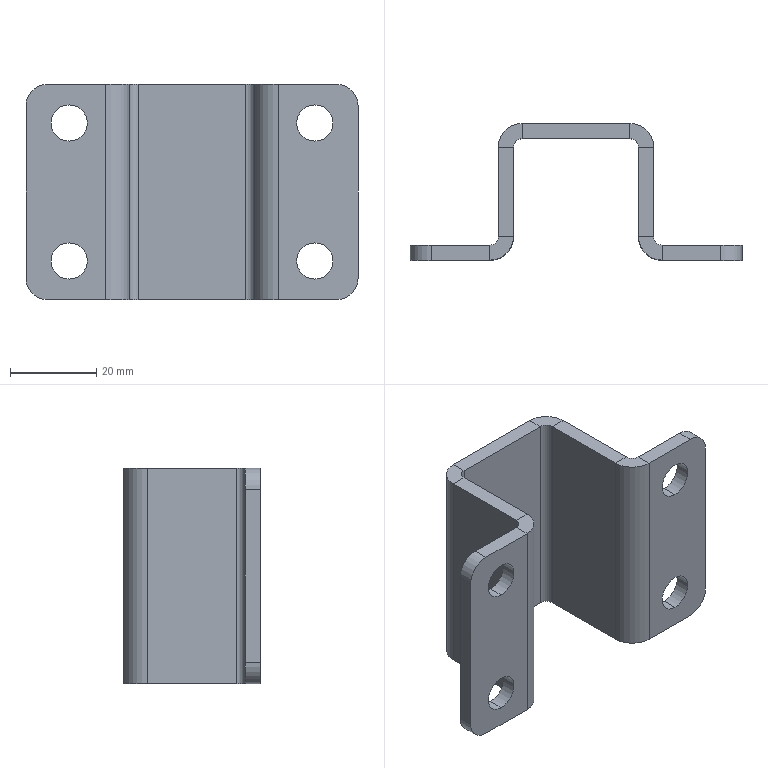Part | STEP file | ABRAZADERA a | 1 solid | 50 faces | box 77 x 31.7 x 50 mm | volume 21367 mm3 | plane 30 | cylinder 20 | commonest cylinder face diameters 8.4 x8 4 x4 10 x4 11 x4
STEP:
#1=CARTESIAN_POINT('',(-28.5,-13.7,11.8));
#2=VERTEX_POINT('',#1);
#3=CARTESIAN_POINT('',(-28.5,-13.7,20.2));
#4=VERTEX_POINT('',#3);
#5=CARTESIAN_POINT('',(-28.5,-13.7,16.));
#6=DIRECTION('',(0.,1.,0.));
#7=DIRECTION('',(-1.,0.,0.));
#8=AXIS2_PLACEMENT_3D('',#5,#6,#7);
#9=CIRCLE('',#8,4.2);
#10=EDGE_CURVE('',#2,#4,#9,.T.);
#11=ORIENTED_EDGE('',*,*,#10,.F.);
#12=CARTESIAN_POINT('',(-28.5,-10.2,11.8));
#13=VERTEX_POINT('',#12);
#14=CARTESIAN_POINT('',(-28.5,-10.2,11.8));
#15=DIRECTION('',(0.,1.,0.));
#16=VECTOR('',#15,1000.);
#17=LINE('',#14,#16);
#18=EDGE_CURVE('',#2,#13,#17,.T.);
#19=ORIENTED_EDGE('',*,*,#18,.T.);
#20=CARTESIAN_POINT('',(-28.5,-10.2,20.2));
#21=VERTEX_POINT('',#20);
#22=CARTESIAN_POINT('',(-28.5,-10.2,16.));
#23=DIRECTION('',(0.,1.,0.));
#24=DIRECTION('',(0.,0.,1.));
#25=AXIS2_PLACEMENT_3D('',#22,#23,#24);
#26=CIRCLE('',#25,4.2);
#27=EDGE_CURVE('',#13,#21,#26,.T.);
#28=ORIENTED_EDGE('',*,*,#27,.T.);
#29=CARTESIAN_POINT('',(-28.5,-10.2,20.2));
#30=DIRECTION('',(0.,1.,0.));
#31=VECTOR('',#30,1000.);
#32=LINE('',#29,#31);
#33=EDGE_CURVE('',#4,#21,#32,.T.);
#34=ORIENTED_EDGE('',*,*,#33,.F.);
#35=EDGE_LOOP('',(#11,#19,#28,#34));
#36=FACE_OUTER_BOUND('',#35,.T.);
#37=CARTESIAN_POINT('',(-28.5,-10.2,16.));
#38=DIRECTION('',(0.,1.,0.));
#39=DIRECTION('',(0.,0.,1.));
#40=AXIS2_PLACEMENT_3D('',#37,#38,#39);
#41=CYLINDRICAL_SURFACE('',#40,4.2);
#42=ADVANCED_FACE('',(#36),#41,.F.);
#43=CARTESIAN_POINT('',(-28.5,-13.7,-20.2));
#44=VERTEX_POINT('',#43);
#45=CARTESIAN_POINT('',(-28.5,-13.7,-11.8));
#46=VERTEX_POINT('',#45);
#47=CARTESIAN_POINT('',(-28.5,-13.7,-16.));
#48=DIRECTION('',(0.,1.,0.));
#49=DIRECTION('',(-1.,0.,0.));
#50=AXIS2_PLACEMENT_3D('',#47,#48,#49);
#51=CIRCLE('',#50,4.2);
#52=EDGE_CURVE('',#44,#46,#51,.T.);
#53=ORIENTED_EDGE('',*,*,#52,.F.);
#54=CARTESIAN_POINT('',(-28.5,-10.2,-20.2));
#55=VERTEX_POINT('',#54);
#56=CARTESIAN_POINT('',(-28.5,-10.2,-20.2));
#57=DIRECTION('',(0.,1.,0.));
#58=VECTOR('',#57,1000.);
#59=LINE('',#56,#58);
#60=EDGE_CURVE('',#44,#55,#59,.T.);
#61=ORIENTED_EDGE('',*,*,#60,.T.);
#62=CARTESIAN_POINT('',(-28.5,-10.2,-11.8));
#63=VERTEX_POINT('',#62);
#64=CARTESIAN_POINT('',(-28.5,-10.2,-16.));
#65=DIRECTION('',(0.,1.,0.));
#66=DIRECTION('',(0.,0.,1.));
#67=AXIS2_PLACEMENT_3D('',#64,#65,#66);
#68=CIRCLE('',#67,4.2);
#69=EDGE_CURVE('',#55,#63,#68,.T.);
#70=ORIENTED_EDGE('',*,*,#69,.T.);
#71=CARTESIAN_POINT('',(-28.5,-10.2,-11.8));
#72=DIRECTION('',(0.,1.,0.));
#73=VECTOR('',#72,1000.);
#74=LINE('',#71,#73);
#75=EDGE_CURVE('',#46,#63,#74,.T.);
#76=ORIENTED_EDGE('',*,*,#75,.F.);
#77=EDGE_LOOP('',(#53,#61,#70,#76));
#78=FACE_OUTER_BOUND('',#77,.T.);
#79=CARTESIAN_POINT('',(-28.5,-10.2,-16.));
#80=DIRECTION('',(0.,1.,0.));
#81=DIRECTION('',(0.,0.,1.));
#82=AXIS2_PLACEMENT_3D('',#79,#80,#81);
#83=CYLINDRICAL_SURFACE('',#82,4.2);
#84=ADVANCED_FACE('',(#78),#83,.F.);
#85=CARTESIAN_POINT('',(28.5,-13.7,11.8));
#86=VERTEX_POINT('',#85);
#87=CARTESIAN_POINT('',(28.5,-13.7,20.2));
#88=VERTEX_POINT('',#87);
#89=CARTESIAN_POINT('',(28.5,-13.7,16.));
#90=DIRECTION('',(0.,1.,0.));
#91=DIRECTION('',(0.,0.,1.));
#92=AXIS2_PLACEMENT_3D('',#89,#90,#91);
#93=CIRCLE('',#92,4.2);
#94=EDGE_CURVE('',#86,#88,#93,.T.);
#95=ORIENTED_EDGE('',*,*,#94,.F.);
#96=CARTESIAN_POINT('',(28.5,-10.2,11.8));
#97=VERTEX_POINT('',#96);
#98=CARTESIAN_POINT('',(28.5,-10.2,11.8));
#99=DIRECTION('',(0.,1.,0.));
#100=VECTOR('',#99,1000.);
#101=LINE('',#98,#100);
#102=EDGE_CURVE('',#86,#97,#101,.T.);
#103=ORIENTED_EDGE('',*,*,#102,.T.);
#104=CARTESIAN_POINT('',(28.5,-10.2,20.2));
#105=VERTEX_POINT('',#104);
#106=CARTESIAN_POINT('',(28.5,-10.2,16.));
#107=DIRECTION('',(0.,1.,0.));
#108=DIRECTION('',(0.,0.,1.));
#109=AXIS2_PLACEMENT_3D('',#106,#107,#108);
#110=CIRCLE('',#109,4.2);
#111=EDGE_CURVE('',#97,#105,#110,.T.);
#112=ORIENTED_EDGE('',*,*,#111,.T.);
#113=CARTESIAN_POINT('',(28.5,-10.2,20.2));
#114=DIRECTION('',(0.,1.,0.));
#115=VECTOR('',#114,1000.);
#116=LINE('',#113,#115);
#117=EDGE_CURVE('',#88,#105,#116,.T.);
#118=ORIENTED_EDGE('',*,*,#117,.F.);
#119=EDGE_LOOP('',(#95,#103,#112,#118));
#120=FACE_OUTER_BOUND('',#119,.T.);
#121=CARTESIAN_POINT('',(28.5,-10.2,16.));
#122=DIRECTION('',(0.,1.,0.));
#123=DIRECTION('',(0.,0.,1.));
#124=AXIS2_PLACEMENT_3D('',#121,#122,#123);
#125=CYLINDRICAL_SURFACE('',#124,4.2);
#126=ADVANCED_FACE('',(#120),#125,.F.);
#127=CARTESIAN_POINT('',(28.5,-13.7,-20.2));
#128=VERTEX_POINT('',#127);
#129=CARTESIAN_POINT('',(28.5,-13.7,-11.8));
#130=VERTEX_POINT('',#129);
#131=CARTESIAN_POINT('',(28.5,-13.7,-16.));
#132=DIRECTION('',(0.,1.,0.));
#133=DIRECTION('',(0.,0.,1.));
#134=AXIS2_PLACEMENT_3D('',#131,#132,#133);
#135=CIRCLE('',#134,4.2);
#136=EDGE_CURVE('',#128,#130,#135,.T.);
#137=ORIENTED_EDGE('',*,*,#136,.F.);
#138=CARTESIAN_POINT('',(28.5,-10.2,-20.2));
#139=VERTEX_POINT('',#138);
#140=CARTESIAN_POINT('',(28.5,-10.2,-20.2));
#141=DIRECTION('',(0.,1.,0.));
#142=VECTOR('',#141,1000.);
#143=LINE('',#140,#142);
#144=EDGE_CURVE('',#128,#139,#143,.T.);
#145=ORIENTED_EDGE('',*,*,#144,.T.);
#146=CARTESIAN_POINT('',(28.5,-10.2,-11.8));
#147=VERTEX_POINT('',#146);
#148=CARTESIAN_POINT('',(28.5,-10.2,-16.));
#149=DIRECTION('',(0.,1.,0.));
#150=DIRECTION('',(0.,0.,1.));
#151=AXIS2_PLACEMENT_3D('',#148,#149,#150);
#152=CIRCLE('',#151,4.2);
#153=EDGE_CURVE('',#139,#147,#152,.T.);
#154=ORIENTED_EDGE('',*,*,#153,.T.);
#155=CARTESIAN_POINT('',(28.5,-10.2,-11.8));
#156=DIRECTION('',(0.,1.,0.));
#157=VECTOR('',#156,1000.);
#158=LINE('',#155,#157);
#159=EDGE_CURVE('',#130,#147,#158,.T.);
#160=ORIENTED_EDGE('',*,*,#159,.F.);
#161=EDGE_LOOP('',(#137,#145,#154,#160));
#162=FACE_OUTER_BOUND('',#161,.T.);
#163=CARTESIAN_POINT('',(28.5,-10.2,-16.));
#164=DIRECTION('',(0.,1.,0.));
#165=DIRECTION('',(0.,0.,1.));
#166=AXIS2_PLACEMENT_3D('',#163,#164,#165);
#167=CYLINDRICAL_SURFACE('',#166,4.2);
#168=ADVANCED_FACE('',(#162),#167,.F.);
#169=CARTESIAN_POINT('',(-20.,-13.7,25.));
#170=VERTEX_POINT('',#169);
#171=CARTESIAN_POINT('',(-20.,-10.2,25.));
#172=VERTEX_POINT('',#171);
#173=CARTESIAN_POINT('',(-20.,-13.7,25.));
#174=DIRECTION('',(0.,1.,0.));
#175=VECTOR('',#174,1000.);
#176=LINE('',#173,#175);
#177=EDGE_CURVE('',#170,#172,#176,.T.);
#178=ORIENTED_EDGE('',*,*,#177,.F.);
#179=CARTESIAN_POINT('',(-14.5,-8.2,25.));
#180=VERTEX_POINT('',#179);
#181=CARTESIAN_POINT('',(-20.,-8.2,25.));
#182=DIRECTION('',(0.,0.,1.));
#183=DIRECTION('',(-1.,0.,0.));
#184=AXIS2_PLACEMENT_3D('',#181,#182,#183);
#185=CIRCLE('',#184,5.5);
#186=EDGE_CURVE('',#170,#180,#185,.T.);
#187=ORIENTED_EDGE('',*,*,#186,.T.);
#188=CARTESIAN_POINT('',(-18.,-8.2,25.));
#189=VERTEX_POINT('',#188);
#190=CARTESIAN_POINT('',(-18.,-8.2,25.));
#191=DIRECTION('',(1.,0.,0.));
#192=VECTOR('',#191,1000.);
#193=LINE('',#190,#192);
#194=EDGE_CURVE('',#189,#180,#193,.T.);
#195=ORIENTED_EDGE('',*,*,#194,.F.);
#196=CARTESIAN_POINT('',(-20.,-8.2,25.));
#197=DIRECTION('',(0.,0.,1.));
#198=DIRECTION('',(1.,0.,0.));
#199=AXIS2_PLACEMENT_3D('',#196,#197,#198);
#200=CIRCLE('',#199,2.);
#201=EDGE_CURVE('',#172,#189,#200,.T.);
#202=ORIENTED_EDGE('',*,*,#201,.F.);
#203=EDGE_LOOP('',(#178,#187,#195,#202));
#204=FACE_OUTER_BOUND('',#203,.T.);
#205=CARTESIAN_POINT('',(-20.,-13.7,25.));
#206=DIRECTION('',(0.,0.,1.));
#207=DIRECTION('',(1.,0.,0.));
#208=AXIS2_PLACEMENT_3D('',#205,#206,#207);
#209=PLANE('',#208);
#210=ADVANCED_FACE('',(#204),#209,.T.);
#211=CARTESIAN_POINT('',(-33.5,-10.2,25.));
#212=VERTEX_POINT('',#211);
#213=CARTESIAN_POINT('',(-14.5,-10.2,25.));
#214=DIRECTION('',(1.,0.,0.));
#215=VECTOR('',#214,1000.);
#216=LINE('',#213,#215);
#217=EDGE_CURVE('',#212,#172,#216,.T.);
#218=ORIENTED_EDGE('',*,*,#217,.F.);
#219=CARTESIAN_POINT('',(-33.5,-13.7,25.));
#220=VERTEX_POINT('',#219);
#221=CARTESIAN_POINT('',(-33.5,-8.2,25.));
#222=DIRECTION('',(0.,-1.,0.));
#223=VECTOR('',#222,1000.);
#224=LINE('',#221,#223);
#225=EDGE_CURVE('',#212,#220,#224,.T.);
#226=ORIENTED_EDGE('',*,*,#225,.T.);
#227=CARTESIAN_POINT('',(-14.5,-13.7,25.));
#228=DIRECTION('',(1.,0.,0.));
#229=VECTOR('',#228,1000.);
#230=LINE('',#227,#229);
#231=EDGE_CURVE('',#220,#170,#230,.T.);
#232=ORIENTED_EDGE('',*,*,#231,.T.);
#233=ORIENTED_EDGE('',*,*,#177,.T.);
#234=EDGE_LOOP('',(#218,#226,#232,#233));
#235=FACE_OUTER_BOUND('',#234,.T.);
#236=CARTESIAN_POINT('',(-18.,-8.2,25.));
#237=DIRECTION('',(0.,0.,1.));
#238=DIRECTION('',(1.,0.,0.));
#239=AXIS2_PLACEMENT_3D('',#236,#237,#238);
#240=PLANE('',#239);
#241=ADVANCED_FACE('',(#235),#240,.T.);
#242=CARTESIAN_POINT('',(-14.5,-8.2,-25.));
#243=VERTEX_POINT('',#242);
#244=CARTESIAN_POINT('',(-18.,-8.2,-25.));
#245=VERTEX_POINT('',#244);
#246=CARTESIAN_POINT('',(-14.5,-8.2,-25.));
#247=DIRECTION('',(-1.,0.,0.));
#248=VECTOR('',#247,1000.);
#249=LINE('',#246,#248);
#250=EDGE_CURVE('',#243,#245,#249,.T.);
#251=ORIENTED_EDGE('',*,*,#250,.F.);
#252=CARTESIAN_POINT('',(-20.,-13.7,-25.));
#253=VERTEX_POINT('',#252);
#254=CARTESIAN_POINT('',(-20.,-8.2,-25.));
#255=DIRECTION('',(0.,0.,1.));
#256=DIRECTION('',(-1.,0.,0.));
#257=AXIS2_PLACEMENT_3D('',#254,#255,#256);
#258=CIRCLE('',#257,5.5);
#259=EDGE_CURVE('',#253,#243,#258,.T.);
#260=ORIENTED_EDGE('',*,*,#259,.F.);
#261=CARTESIAN_POINT('',(-20.,-10.2,-25.));
#262=VERTEX_POINT('',#261);
#263=CARTESIAN_POINT('',(-20.,-10.2,-25.));
#264=DIRECTION('',(0.,-1.,0.));
#265=VECTOR('',#264,1000.);
#266=LINE('',#263,#265);
#267=EDGE_CURVE('',#262,#253,#266,.T.);
#268=ORIENTED_EDGE('',*,*,#267,.F.);
#269=CARTESIAN_POINT('',(-20.,-8.2,-25.));
#270=DIRECTION('',(0.,0.,1.));
#271=DIRECTION('',(1.,0.,0.));
#272=AXIS2_PLACEMENT_3D('',#269,#270,#271);
#273=CIRCLE('',#272,2.);
#274=EDGE_CURVE('',#262,#245,#273,.T.);
#275=ORIENTED_EDGE('',*,*,#274,.T.);
#276=EDGE_LOOP('',(#251,#260,#268,#275));
#277=FACE_OUTER_BOUND('',#276,.T.);
#278=CARTESIAN_POINT('',(-14.5,-8.2,-25.));
#279=DIRECTION('',(0.,0.,-1.));
#280=DIRECTION('',(-1.,0.,0.));
#281=AXIS2_PLACEMENT_3D('',#278,#279,#280);
#282=PLANE('',#281);
#283=ADVANCED_FACE('',(#277),#282,.T.);
#284=CARTESIAN_POINT('',(-14.5,12.5,-25.));
#285=VERTEX_POINT('',#284);
#286=CARTESIAN_POINT('',(-14.5,14.5,-25.));
#287=DIRECTION('',(0.,1.,0.));
#288=VECTOR('',#287,1000.);
#289=LINE('',#286,#288);
#290=EDGE_CURVE('',#243,#285,#289,.T.);
#291=ORIENTED_EDGE('',*,*,#290,.F.);
#292=ORIENTED_EDGE('',*,*,#250,.T.);
#293=CARTESIAN_POINT('',(-18.,12.5,-25.));
#294=VERTEX_POINT('',#293);
#295=CARTESIAN_POINT('',(-18.,14.5,-25.));
#296=DIRECTION('',(0.,1.,0.));
#297=VECTOR('',#296,1000.);
#298=LINE('',#295,#297);
#299=EDGE_CURVE('',#245,#294,#298,.T.);
#300=ORIENTED_EDGE('',*,*,#299,.T.);
#301=CARTESIAN_POINT('',(-18.,12.5,-25.));
#302=DIRECTION('',(1.,0.,0.));
#303=VECTOR('',#302,1000.);
#304=LINE('',#301,#303);
#305=EDGE_CURVE('',#294,#285,#304,.T.);
#306=ORIENTED_EDGE('',*,*,#305,.T.);
#307=EDGE_LOOP('',(#291,#292,#300,#306));
#308=FACE_OUTER_BOUND('',#307,.T.);
#309=CARTESIAN_POINT('',(-20.,-10.2,-25.));
#310=DIRECTION('',(0.,0.,-1.));
#311=DIRECTION('',(-1.,0.,0.));
#312=AXIS2_PLACEMENT_3D('',#309,#310,#311);
#313=PLANE('',#312);
#314=ADVANCED_FACE('',(#308),#313,.T.);
#315=CARTESIAN_POINT('',(-14.5,12.5,25.));
#316=VERTEX_POINT('',#315);
#317=CARTESIAN_POINT('',(-18.,12.5,25.));
#318=VERTEX_POINT('',#317);
#319=CARTESIAN_POINT('',(-14.5,12.5,25.));
#320=DIRECTION('',(-1.,0.,0.));
#321=VECTOR('',#320,1000.);
#322=LINE('',#319,#321);
#323=EDGE_CURVE('',#316,#318,#322,.T.);
#324=ORIENTED_EDGE('',*,*,#323,.F.);
#325=CARTESIAN_POINT('',(-12.5,14.5,25.));
#326=VERTEX_POINT('',#325);
#327=CARTESIAN_POINT('',(-12.5,12.5,25.));
#328=DIRECTION('',(0.,0.,-1.));
#329=DIRECTION('',(1.,0.,0.));
#330=AXIS2_PLACEMENT_3D('',#327,#328,#329);
#331=CIRCLE('',#330,2.);
#332=EDGE_CURVE('',#316,#326,#331,.T.);
#333=ORIENTED_EDGE('',*,*,#332,.T.);
#334=CARTESIAN_POINT('',(-12.5,18.,25.));
#335=VERTEX_POINT('',#334);
#336=CARTESIAN_POINT('',(-12.5,18.,25.));
#337=DIRECTION('',(0.,-1.,0.));
#338=VECTOR('',#337,1000.);
#339=LINE('',#336,#338);
#340=EDGE_CURVE('',#335,#326,#339,.T.);
#341=ORIENTED_EDGE('',*,*,#340,.F.);
#342=CARTESIAN_POINT('',(-12.5,12.5,25.));
#343=DIRECTION('',(0.,0.,-1.));
#344=DIRECTION('',(1.,0.,0.));
#345=AXIS2_PLACEMENT_3D('',#342,#343,#344);
#346=CIRCLE('',#345,5.5);
#347=EDGE_CURVE('',#318,#335,#346,.T.);
#348=ORIENTED_EDGE('',*,*,#347,.F.);
#349=EDGE_LOOP('',(#324,#333,#341,#348));
#350=FACE_OUTER_BOUND('',#349,.T.);
#351=CARTESIAN_POINT('',(-14.5,12.5,25.));
#352=DIRECTION('',(0.,0.,1.));
#353=DIRECTION('',(1.,0.,0.));
#354=AXIS2_PLACEMENT_3D('',#351,#352,#353);
#355=PLANE('',#354);
#356=ADVANCED_FACE('',(#350),#355,.T.);
#357=CARTESIAN_POINT('',(-14.5,14.5,25.));
#358=DIRECTION('',(0.,1.,0.));
#359=VECTOR('',#358,1000.);
#360=LINE('',#357,#359);
#361=EDGE_CURVE('',#180,#316,#360,.T.);
#362=ORIENTED_EDGE('',*,*,#361,.T.);
#363=ORIENTED_EDGE('',*,*,#323,.T.);
#364=CARTESIAN_POINT('',(-18.,14.5,25.));
#365=DIRECTION('',(0.,1.,0.));
#366=VECTOR('',#365,1000.);
#367=LINE('',#364,#366);
#368=EDGE_CURVE('',#189,#318,#367,.T.);
#369=ORIENTED_EDGE('',*,*,#368,.F.);
#370=ORIENTED_EDGE('',*,*,#194,.T.);
#371=EDGE_LOOP('',(#362,#363,#369,#370));
#372=FACE_OUTER_BOUND('',#371,.T.);
#373=CARTESIAN_POINT('',(-12.5,18.,25.));
#374=DIRECTION('',(0.,0.,1.));
#375=DIRECTION('',(1.,0.,0.));
#376=AXIS2_PLACEMENT_3D('',#373,#374,#375);
#377=PLANE('',#376);
#378=ADVANCED_FACE('',(#372),#377,.T.);
#379=CARTESIAN_POINT('',(-12.5,14.5,-25.));
#380=VERTEX_POINT('',#379);
#381=CARTESIAN_POINT('',(-12.5,18.,-25.));
#382=VERTEX_POINT('',#381);
#383=CARTESIAN_POINT('',(-12.5,14.5,-25.));
#384=DIRECTION('',(0.,1.,0.));
#385=VECTOR('',#384,1000.);
#386=LINE('',#383,#385);
#387=EDGE_CURVE('',#380,#382,#386,.T.);
#388=ORIENTED_EDGE('',*,*,#387,.F.);
#389=CARTESIAN_POINT('',(-12.5,12.5,-25.));
#390=DIRECTION('',(0.,0.,-1.));
#391=DIRECTION('',(1.,0.,0.));
#392=AXIS2_PLACEMENT_3D('',#389,#390,#391);
#393=CIRCLE('',#392,2.);
#394=EDGE_CURVE('',#285,#380,#393,.T.);
#395=ORIENTED_EDGE('',*,*,#394,.F.);
#396=ORIENTED_EDGE('',*,*,#305,.F.);
#397=CARTESIAN_POINT('',(-12.5,12.5,-25.));
#398=DIRECTION('',(0.,0.,-1.));
#399=DIRECTION('',(1.,0.,0.));
#400=AXIS2_PLACEMENT_3D('',#397,#398,#399);
#401=CIRCLE('',#400,5.5);
#402=EDGE_CURVE('',#294,#382,#401,.T.);
#403=ORIENTED_EDGE('',*,*,#402,.T.);
#404=EDGE_LOOP('',(#388,#395,#396,#403));
#405=FACE_OUTER_BOUND('',#404,.T.);
#406=CARTESIAN_POINT('',(-12.5,14.5,-25.));
#407=DIRECTION('',(0.,0.,-1.));
#408=DIRECTION('',(-1.,0.,0.));
#409=AXIS2_PLACEMENT_3D('',#406,#407,#408);
#410=PLANE('',#409);
#411=ADVANCED_FACE('',(#405),#410,.T.);
#412=CARTESIAN_POINT('',(12.5,14.5,-25.));
#413=VERTEX_POINT('',#412);
#414=CARTESIAN_POINT('',(-14.5,14.5,-25.));
#415=DIRECTION('',(1.,0.,0.));
#416=VECTOR('',#415,1000.);
#417=LINE('',#414,#416);
#418=EDGE_CURVE('',#380,#413,#417,.T.);
#419=ORIENTED_EDGE('',*,*,#418,.F.);
#420=ORIENTED_EDGE('',*,*,#387,.T.);
#421=CARTESIAN_POINT('',(12.5,18.,-25.));
#422=VERTEX_POINT('',#421);
#423=CARTESIAN_POINT('',(-14.5,18.,-25.));
#424=DIRECTION('',(1.,0.,0.));
#425=VECTOR('',#424,1000.);
#426=LINE('',#423,#425);
#427=EDGE_CURVE('',#382,#422,#426,.T.);
#428=ORIENTED_EDGE('',*,*,#427,.T.);
#429=CARTESIAN_POINT('',(12.5,18.,-25.));
#430=DIRECTION('',(0.,-1.,0.));
#431=VECTOR('',#430,1000.);
#432=LINE('',#429,#431);
#433=EDGE_CURVE('',#422,#413,#432,.T.);
#434=ORIENTED_EDGE('',*,*,#433,.T.);
#435=EDGE_LOOP('',(#419,#420,#428,#434));
#436=FACE_OUTER_BOUND('',#435,.T.);
#437=CARTESIAN_POINT('',(-18.,12.5,-25.));
#438=DIRECTION('',(0.,0.,-1.));
#439=DIRECTION('',(-1.,0.,0.));
#440=AXIS2_PLACEMENT_3D('',#437,#438,#439);
#441=PLANE('',#440);
#442=ADVANCED_FACE('',(#436),#441,.T.);
#443=CARTESIAN_POINT('',(12.5,14.5,25.));
#444=VERTEX_POINT('',#443);
#445=CARTESIAN_POINT('',(12.5,18.,25.));
#446=VERTEX_POINT('',#445);
#447=CARTESIAN_POINT('',(12.5,14.5,25.));
#448=DIRECTION('',(0.,1.,0.));
#449=VECTOR('',#448,1000.);
#450=LINE('',#447,#449);
#451=EDGE_CURVE('',#444,#446,#450,.T.);
#452=ORIENTED_EDGE('',*,*,#451,.F.);
#453=CARTESIAN_POINT('',(14.5,12.5,25.));
#454=VERTEX_POINT('',#453);
#455=CARTESIAN_POINT('',(12.5,12.5,25.));
#456=DIRECTION('',(0.,0.,-1.));
#457=DIRECTION('',(1.,0.,0.));
#458=AXIS2_PLACEMENT_3D('',#455,#456,#457);
#459=CIRCLE('',#458,2.);
#460=EDGE_CURVE('',#444,#454,#459,.T.);
#461=ORIENTED_EDGE('',*,*,#460,.T.);
#462=CARTESIAN_POINT('',(18.,12.5,25.));
#463=VERTEX_POINT('',#462);
#464=CARTESIAN_POINT('',(18.,12.5,25.));
#465=DIRECTION('',(-1.,0.,0.));
#466=VECTOR('',#465,1000.);
#467=LINE('',#464,#466);
#468=EDGE_CURVE('',#463,#454,#467,.T.);
#469=ORIENTED_EDGE('',*,*,#468,.F.);
#470=CARTESIAN_POINT('',(12.5,12.5,25.));
#471=DIRECTION('',(0.,0.,-1.));
#472=DIRECTION('',(1.,0.,0.));
#473=AXIS2_PLACEMENT_3D('',#470,#471,#472);
#474=CIRCLE('',#473,5.5);
#475=EDGE_CURVE('',#446,#463,#474,.T.);
#476=ORIENTED_EDGE('',*,*,#475,.F.);
#477=EDGE_LOOP('',(#452,#461,#469,#476));
#478=FACE_OUTER_BOUND('',#477,.T.);
#479=CARTESIAN_POINT('',(12.5,14.5,25.));
#480=DIRECTION('',(0.,0.,1.));
#481=DIRECTION('',(1.,0.,0.));
#482=AXIS2_PLACEMENT_3D('',#479,#480,#481);
#483=PLANE('',#482);
#484=ADVANCED_FACE('',(#478),#483,.T.);
#485=CARTESIAN_POINT('',(-14.5,14.5,25.));
#486=DIRECTION('',(1.,0.,0.));
#487=VECTOR('',#486,1000.);
#488=LINE('',#485,#487);
#489=EDGE_CURVE('',#326,#444,#488,.T.);
#490=ORIENTED_EDGE('',*,*,#489,.T.);
#491=ORIENTED_EDGE('',*,*,#451,.T.);
#492=CARTESIAN_POINT('',(-14.5,18.,25.));
#493=DIRECTION('',(1.,0.,0.));
#494=VECTOR('',#493,1000.);
#495=LINE('',#492,#494);
#496=EDGE_CURVE('',#335,#446,#495,.T.);
#497=ORIENTED_EDGE('',*,*,#496,.F.);
#498=ORIENTED_EDGE('',*,*,#340,.T.);
#499=EDGE_LOOP('',(#490,#491,#497,#498));
#500=FACE_OUTER_BOUND('',#499,.T.);
#501=CARTESIAN_POINT('',(18.,12.5,25.));
#502=DIRECTION('',(0.,0.,1.));
#503=DIRECTION('',(1.,0.,0.));
#504=AXIS2_PLACEMENT_3D('',#501,#502,#503);
#505=PLANE('',#504);
#506=ADVANCED_FACE('',(#500),#505,.T.);
#507=CARTESIAN_POINT('',(14.5,12.5,-25.));
#508=VERTEX_POINT('',#507);
#509=CARTESIAN_POINT('',(18.,12.5,-25.));
#510=VERTEX_POINT('',#509);
#511=CARTESIAN_POINT('',(14.5,12.5,-25.));
#512=DIRECTION('',(1.,0.,0.));
#513=VECTOR('',#512,1000.);
#514=LINE('',#511,#513);
#515=EDGE_CURVE('',#508,#510,#514,.T.);
#516=ORIENTED_EDGE('',*,*,#515,.F.);
#517=CARTESIAN_POINT('',(12.5,12.5,-25.));
#518=DIRECTION('',(0.,0.,-1.));
#519=DIRECTION('',(1.,0.,0.));
#520=AXIS2_PLACEMENT_3D('',#517,#518,#519);
#521=CIRCLE('',#520,2.);
#522=EDGE_CURVE('',#413,#508,#521,.T.);
#523=ORIENTED_EDGE('',*,*,#522,.F.);
#524=ORIENTED_EDGE('',*,*,#433,.F.);
#525=CARTESIAN_POINT('',(12.5,12.5,-25.));
#526=DIRECTION('',(0.,0.,-1.));
#527=DIRECTION('',(1.,0.,0.));
#528=AXIS2_PLACEMENT_3D('',#525,#526,#527);
#529=CIRCLE('',#528,5.5);
#530=EDGE_CURVE('',#422,#510,#529,.T.);
#531=ORIENTED_EDGE('',*,*,#530,.T.);
#532=EDGE_LOOP('',(#516,#523,#524,#531));
#533=FACE_OUTER_BOUND('',#532,.T.);
#534=CARTESIAN_POINT('',(14.5,12.5,-25.));
#535=DIRECTION('',(0.,0.,-1.));
#536=DIRECTION('',(-1.,0.,0.));
#537=AXIS2_PLACEMENT_3D('',#534,#535,#536);
#538=PLANE('',#537);
#539=ADVANCED_FACE('',(#533),#538,.T.);
#540=CARTESIAN_POINT('',(14.5,-8.2,-25.));
#541=VERTEX_POINT('',#540);
#542=CARTESIAN_POINT('',(14.5,14.5,-25.));
#543=DIRECTION('',(0.,-1.,0.));
#544=VECTOR('',#543,1000.);
#545=LINE('',#542,#544);
#546=EDGE_CURVE('',#508,#541,#545,.T.);
#547=ORIENTED_EDGE('',*,*,#546,.F.);
#548=ORIENTED_EDGE('',*,*,#515,.T.);
#549=CARTESIAN_POINT('',(18.,-8.2,-25.));
#550=VERTEX_POINT('',#549);
#551=CARTESIAN_POINT('',(18.,14.5,-25.));
#552=DIRECTION('',(0.,-1.,0.));
#553=VECTOR('',#552,1000.);
#554=LINE('',#551,#553);
#555=EDGE_CURVE('',#510,#550,#554,.T.);
#556=ORIENTED_EDGE('',*,*,#555,.T.);
#557=CARTESIAN_POINT('',(18.,-8.2,-25.));
#558=DIRECTION('',(-1.,0.,0.));
#559=VECTOR('',#558,1000.);
#560=LINE('',#557,#559);
#561=EDGE_CURVE('',#550,#541,#560,.T.);
#562=ORIENTED_EDGE('',*,*,#561,.T.);
#563=EDGE_LOOP('',(#547,#548,#556,#562));
#564=FACE_OUTER_BOUND('',#563,.T.);
#565=CARTESIAN_POINT('',(12.5,18.,-25.));
#566=DIRECTION('',(0.,0.,-1.));
#567=DIRECTION('',(-1.,0.,0.));
#568=AXIS2_PLACEMENT_3D('',#565,#566,#567);
#569=PLANE('',#568);
#570=ADVANCED_FACE('',(#564),#569,.T.);
#571=CARTESIAN_POINT('',(14.5,-8.2,25.));
#572=VERTEX_POINT('',#571);
#573=CARTESIAN_POINT('',(18.,-8.2,25.));
#574=VERTEX_POINT('',#573);
#575=CARTESIAN_POINT('',(14.5,-8.2,25.));
#576=DIRECTION('',(1.,0.,0.));
#577=VECTOR('',#576,1000.);
#578=LINE('',#575,#577);
#579=EDGE_CURVE('',#572,#574,#578,.T.);
#580=ORIENTED_EDGE('',*,*,#579,.F.);
#581=CARTESIAN_POINT('',(20.,-13.7,25.));
#582=VERTEX_POINT('',#581);
#583=CARTESIAN_POINT('',(20.,-8.2,25.));
#584=DIRECTION('',(0.,0.,1.));
#585=DIRECTION('',(-1.,0.,0.));
#586=AXIS2_PLACEMENT_3D('',#583,#584,#585);
#587=CIRCLE('',#586,5.5);
#588=EDGE_CURVE('',#572,#582,#587,.T.);
#589=ORIENTED_EDGE('',*,*,#588,.T.);
#590=CARTESIAN_POINT('',(20.,-10.2,25.));
#591=VERTEX_POINT('',#590);
#592=CARTESIAN_POINT('',(20.,-10.2,25.));
#593=DIRECTION('',(0.,-1.,0.));
#594=VECTOR('',#593,1000.);
#595=LINE('',#592,#594);
#596=EDGE_CURVE('',#591,#582,#595,.T.);
#597=ORIENTED_EDGE('',*,*,#596,.F.);
#598=CARTESIAN_POINT('',(20.,-8.2,25.));
#599=DIRECTION('',(0.,0.,1.));
#600=DIRECTION('',(1.,0.,0.));
#601=AXIS2_PLACEMENT_3D('',#598,#599,#600);
#602=CIRCLE('',#601,2.);
#603=EDGE_CURVE('',#574,#591,#602,.T.);
#604=ORIENTED_EDGE('',*,*,#603,.F.);
#605=EDGE_LOOP('',(#580,#589,#597,#604));
#606=FACE_OUTER_BOUND('',#605,.T.);
#607=CARTESIAN_POINT('',(14.5,-8.2,25.));
#608=DIRECTION('',(0.,0.,1.));
#609=DIRECTION('',(1.,0.,0.));
#610=AXIS2_PLACEMENT_3D('',#607,#608,#609);
#611=PLANE('',#610);
#612=ADVANCED_FACE('',(#606),#611,.T.);
#613=CARTESIAN_POINT('',(14.5,14.5,25.));
#614=DIRECTION('',(0.,-1.,0.));
#615=VECTOR('',#614,1000.);
#616=LINE('',#613,#615);
#617=EDGE_CURVE('',#454,#572,#616,.T.);
#618=ORIENTED_EDGE('',*,*,#617,.T.);
#619=ORIENTED_EDGE('',*,*,#579,.T.);
#620=CARTESIAN_POINT('',(18.,14.5,25.));
#621=DIRECTION('',(0.,-1.,0.));
#622=VECTOR('',#621,1000.);
#623=LINE('',#620,#622);
#624=EDGE_CURVE('',#463,#574,#623,.T.);
#625=ORIENTED_EDGE('',*,*,#624,.F.);
#626=ORIENTED_EDGE('',*,*,#468,.T.);
#627=EDGE_LOOP('',(#618,#619,#625,#626));
#628=FACE_OUTER_BOUND('',#627,.T.);
#629=CARTESIAN_POINT('',(20.,-10.2,25.));
#630=DIRECTION('',(0.,0.,1.));
#631=DIRECTION('',(1.,0.,0.));
#632=AXIS2_PLACEMENT_3D('',#629,#630,#631);
#633=PLANE('',#632);
#634=ADVANCED_FACE('',(#628),#633,.T.);
#635=CARTESIAN_POINT('',(20.,-13.7,-25.));
#636=VERTEX_POINT('',#635);
#637=CARTESIAN_POINT('',(20.,-10.2,-25.));
#638=VERTEX_POINT('',#637);
#639=CARTESIAN_POINT('',(20.,-13.7,-25.));
#640=DIRECTION('',(0.,1.,0.));
#641=VECTOR('',#640,1000.);
#642=LINE('',#639,#641);
#643=EDGE_CURVE('',#636,#638,#642,.T.);
#644=ORIENTED_EDGE('',*,*,#643,.F.);
#645=CARTESIAN_POINT('',(20.,-8.2,-25.));
#646=DIRECTION('',(0.,0.,1.));
#647=DIRECTION('',(-1.,0.,0.));
#648=AXIS2_PLACEMENT_3D('',#645,#646,#647);
#649=CIRCLE('',#648,5.5);
#650=EDGE_CURVE('',#541,#636,#649,.T.);
#651=ORIENTED_EDGE('',*,*,#650,.F.);
#652=ORIENTED_EDGE('',*,*,#561,.F.);
#653=CARTESIAN_POINT('',(20.,-8.2,-25.));
#654=DIRECTION('',(0.,0.,1.));
#655=DIRECTION('',(1.,0.,0.));
#656=AXIS2_PLACEMENT_3D('',#653,#654,#655);
#657=CIRCLE('',#656,2.);
#658=EDGE_CURVE('',#550,#638,#657,.T.);
#659=ORIENTED_EDGE('',*,*,#658,.T.);
#660=EDGE_LOOP('',(#644,#651,#652,#659));
#661=FACE_OUTER_BOUND('',#660,.T.);
#662=CARTESIAN_POINT('',(20.,-13.7,-25.));
#663=DIRECTION('',(0.,0.,-1.));
#664=DIRECTION('',(-1.,0.,0.));
#665=AXIS2_PLACEMENT_3D('',#662,#663,#664);
#666=PLANE('',#665);
#667=ADVANCED_FACE('',(#661),#666,.T.);
#668=CARTESIAN_POINT('',(33.5,-10.2,-25.));
#669=VERTEX_POINT('',#668);
#670=CARTESIAN_POINT('',(14.5,-10.2,-25.));
#671=DIRECTION('',(1.,0.,0.));
#672=VECTOR('',#671,1000.);
#673=LINE('',#670,#672);
#674=EDGE_CURVE('',#638,#669,#673,.T.);
#675=ORIENTED_EDGE('',*,*,#674,.T.);
#676=CARTESIAN_POINT('',(33.5,-13.7,-25.));
#677=VERTEX_POINT('',#676);
#678=CARTESIAN_POINT('',(33.5,-8.2,-25.));
#679=DIRECTION('',(0.,-1.,0.));
#680=VECTOR('',#679,1000.);
#681=LINE('',#678,#680);
#682=EDGE_CURVE('',#669,#677,#681,.T.);
#683=ORIENTED_EDGE('',*,*,#682,.T.);
#684=CARTESIAN_POINT('',(14.5,-13.7,-25.));
#685=DIRECTION('',(1.,0.,0.));
#686=VECTOR('',#685,1000.);
#687=LINE('',#684,#686);
#688=EDGE_CURVE('',#636,#677,#687,.T.);
#689=ORIENTED_EDGE('',*,*,#688,.F.);
#690=ORIENTED_EDGE('',*,*,#643,.T.);
#691=EDGE_LOOP('',(#675,#683,#689,#690));
#692=FACE_OUTER_BOUND('',#691,.T.);
#693=CARTESIAN_POINT('',(18.,-8.2,-25.));
#694=DIRECTION('',(0.,0.,-1.));
#695=DIRECTION('',(-1.,0.,0.));
#696=AXIS2_PLACEMENT_3D('',#693,#694,#695);
#697=PLANE('',#696);
#698=ADVANCED_FACE('',(#692),#697,.T.);
#699=CARTESIAN_POINT('',(28.5,-13.7,16.));
#700=DIRECTION('',(0.,1.,0.));
#701=DIRECTION('',(0.,0.,1.));
#702=AXIS2_PLACEMENT_3D('',#699,#700,#701);
#703=CIRCLE('',#702,4.2);
#704=EDGE_CURVE('',#88,#86,#703,.T.);
#705=ORIENTED_EDGE('',*,*,#704,.T.);
#706=ORIENTED_EDGE('',*,*,#94,.T.);
#707=EDGE_LOOP('',(#705,#706));
#708=FACE_BOUND('',#707,.T.);
#709=CARTESIAN_POINT('',(28.5,-13.7,-16.));
#710=DIRECTION('',(0.,1.,0.));
#711=DIRECTION('',(0.,0.,1.));
#712=AXIS2_PLACEMENT_3D('',#709,#710,#711);
#713=CIRCLE('',#712,4.2);
#714=EDGE_CURVE('',#130,#128,#713,.T.);
#715=ORIENTED_EDGE('',*,*,#714,.T.);
#716=ORIENTED_EDGE('',*,*,#136,.T.);
#717=EDGE_LOOP('',(#715,#716));
#718=FACE_BOUND('',#717,.T.);
#719=ORIENTED_EDGE('',*,*,#688,.T.);
#720=CARTESIAN_POINT('',(38.5,-13.7,-20.));
#721=VERTEX_POINT('',#720);
#722=CARTESIAN_POINT('',(33.5,-13.7,-20.));
#723=DIRECTION('',(0.,-1.,0.));
#724=DIRECTION('',(0.,0.,1.));
#725=AXIS2_PLACEMENT_3D('',#722,#723,#724);
#726=CIRCLE('',#725,5.);
#727=EDGE_CURVE('',#677,#721,#726,.T.);
#728=ORIENTED_EDGE('',*,*,#727,.T.);
#729=CARTESIAN_POINT('',(38.5,-13.7,20.));
#730=VERTEX_POINT('',#729);
#731=CARTESIAN_POINT('',(38.5,-13.7,25.));
#732=DIRECTION('',(0.,0.,-1.));
#733=VECTOR('',#732,1000.);
#734=LINE('',#731,#733);
#735=EDGE_CURVE('',#730,#721,#734,.T.);
#736=ORIENTED_EDGE('',*,*,#735,.F.);
#737=CARTESIAN_POINT('',(33.5,-13.7,25.));
#738=VERTEX_POINT('',#737);
#739=CARTESIAN_POINT('',(33.5,-13.7,20.));
#740=DIRECTION('',(0.,-1.,0.));
#741=DIRECTION('',(0.,0.,1.));
#742=AXIS2_PLACEMENT_3D('',#739,#740,#741);
#743=CIRCLE('',#742,5.);
#744=EDGE_CURVE('',#730,#738,#743,.T.);
#745=ORIENTED_EDGE('',*,*,#744,.T.);
#746=CARTESIAN_POINT('',(14.5,-13.7,25.));
#747=DIRECTION('',(1.,0.,0.));
#748=VECTOR('',#747,1000.);
#749=LINE('',#746,#748);
#750=EDGE_CURVE('',#582,#738,#749,.T.);
#751=ORIENTED_EDGE('',*,*,#750,.F.);
#752=CARTESIAN_POINT('',(20.,-13.7,25.));
#753=DIRECTION('',(0.,0.,-1.));
#754=VECTOR('',#753,1000.);
#755=LINE('',#752,#754);
#756=EDGE_CURVE('',#582,#636,#755,.T.);
#757=ORIENTED_EDGE('',*,*,#756,.T.);
#758=EDGE_LOOP('',(#719,#728,#736,#745,#751,#757));
#759=FACE_OUTER_BOUND('',#758,.T.);
#760=CARTESIAN_POINT('',(14.5,-13.7,25.));
#761=DIRECTION('',(0.,1.,0.));
#762=DIRECTION('',(0.,0.,1.));
#763=AXIS2_PLACEMENT_3D('',#760,#761,#762);
#764=PLANE('',#763);
#765=ADVANCED_FACE('',(#708,#718,#759),#764,.F.);
#766=ORIENTED_EDGE('',*,*,#735,.T.);
#767=CARTESIAN_POINT('',(38.5,-10.2,-20.));
#768=VERTEX_POINT('',#767);
#769=CARTESIAN_POINT('',(38.5,-10.2,-20.));
#770=DIRECTION('',(0.,1.,0.));
#771=VECTOR('',#770,1000.);
#772=LINE('',#769,#771);
#773=EDGE_CURVE('',#721,#768,#772,.T.);
#774=ORIENTED_EDGE('',*,*,#773,.T.);
#775=CARTESIAN_POINT('',(38.5,-10.2,20.));
#776=VERTEX_POINT('',#775);
#777=CARTESIAN_POINT('',(38.5,-10.2,25.));
#778=DIRECTION('',(0.,0.,-1.));
#779=VECTOR('',#778,1000.);
#780=LINE('',#777,#779);
#781=EDGE_CURVE('',#776,#768,#780,.T.);
#782=ORIENTED_EDGE('',*,*,#781,.F.);
#783=CARTESIAN_POINT('',(38.5,-10.2,20.));
#784=DIRECTION('',(0.,-1.,0.));
#785=VECTOR('',#784,1000.);
#786=LINE('',#783,#785);
#787=EDGE_CURVE('',#776,#730,#786,.T.);
#788=ORIENTED_EDGE('',*,*,#787,.T.);
#789=EDGE_LOOP('',(#766,#774,#782,#788));
#790=FACE_OUTER_BOUND('',#789,.T.);
#791=CARTESIAN_POINT('',(38.5,-10.2,25.));
#792=DIRECTION('',(1.,0.,0.));
#793=DIRECTION('',(0.,1.,0.));
#794=AXIS2_PLACEMENT_3D('',#791,#792,#793);
#795=PLANE('',#794);
#796=ADVANCED_FACE('',(#790),#795,.T.);
#797=CARTESIAN_POINT('',(28.5,-10.2,16.));
#798=DIRECTION('',(0.,1.,0.));
#799=DIRECTION('',(0.,0.,1.));
#800=AXIS2_PLACEMENT_3D('',#797,#798,#799);
#801=CIRCLE('',#800,4.2);
#802=EDGE_CURVE('',#105,#97,#801,.T.);
#803=ORIENTED_EDGE('',*,*,#802,.F.);
#804=ORIENTED_EDGE('',*,*,#111,.F.);
#805=EDGE_LOOP('',(#803,#804));
#806=FACE_BOUND('',#805,.T.);
#807=CARTESIAN_POINT('',(28.5,-10.2,-16.));
#808=DIRECTION('',(0.,1.,0.));
#809=DIRECTION('',(0.,0.,1.));
#810=AXIS2_PLACEMENT_3D('',#807,#808,#809);
#811=CIRCLE('',#810,4.2);
#812=EDGE_CURVE('',#147,#139,#811,.T.);
#813=ORIENTED_EDGE('',*,*,#812,.F.);
#814=ORIENTED_EDGE('',*,*,#153,.F.);
#815=EDGE_LOOP('',(#813,#814));
#816=FACE_BOUND('',#815,.T.);
#817=ORIENTED_EDGE('',*,*,#781,.T.);
#818=CARTESIAN_POINT('',(33.5,-10.2,-20.));
#819=DIRECTION('',(0.,1.,0.));
#820=DIRECTION('',(0.,0.,1.));
#821=AXIS2_PLACEMENT_3D('',#818,#819,#820);
#822=CIRCLE('',#821,5.);
#823=EDGE_CURVE('',#768,#669,#822,.T.);
#824=ORIENTED_EDGE('',*,*,#823,.T.);
#825=ORIENTED_EDGE('',*,*,#674,.F.);
#826=CARTESIAN_POINT('',(20.,-10.2,25.));
#827=DIRECTION('',(0.,0.,-1.));
#828=VECTOR('',#827,1000.);
#829=LINE('',#826,#828);
#830=EDGE_CURVE('',#591,#638,#829,.T.);
#831=ORIENTED_EDGE('',*,*,#830,.F.);
#832=CARTESIAN_POINT('',(33.5,-10.2,25.));
#833=VERTEX_POINT('',#832);
#834=CARTESIAN_POINT('',(14.5,-10.2,25.));
#835=DIRECTION('',(1.,0.,0.));
#836=VECTOR('',#835,1000.);
#837=LINE('',#834,#836);
#838=EDGE_CURVE('',#591,#833,#837,.T.);
#839=ORIENTED_EDGE('',*,*,#838,.T.);
#840=CARTESIAN_POINT('',(33.5,-10.2,20.));
#841=DIRECTION('',(0.,1.,0.));
#842=DIRECTION('',(0.,0.,1.));
#843=AXIS2_PLACEMENT_3D('',#840,#841,#842);
#844=CIRCLE('',#843,5.);
#845=EDGE_CURVE('',#833,#776,#844,.T.);
#846=ORIENTED_EDGE('',*,*,#845,.T.);
#847=EDGE_LOOP('',(#817,#824,#825,#831,#839,#846));
#848=FACE_OUTER_BOUND('',#847,.T.);
#849=CARTESIAN_POINT('',(14.5,-10.2,25.));
#850=DIRECTION('',(0.,1.,0.));
#851=DIRECTION('',(0.,0.,1.));
#852=AXIS2_PLACEMENT_3D('',#849,#850,#851);
#853=PLANE('',#852);
#854=ADVANCED_FACE('',(#806,#816,#848),#853,.T.);
#855=ORIENTED_EDGE('',*,*,#658,.F.);
#856=CARTESIAN_POINT('',(18.,-8.2,25.));
#857=DIRECTION('',(0.,0.,-1.));
#858=VECTOR('',#857,1000.);
#859=LINE('',#856,#858);
#860=EDGE_CURVE('',#574,#550,#859,.T.);
#861=ORIENTED_EDGE('',*,*,#860,.F.);
#862=ORIENTED_EDGE('',*,*,#603,.T.);
#863=ORIENTED_EDGE('',*,*,#830,.T.);
#864=EDGE_LOOP('',(#855,#861,#862,#863));
#865=FACE_OUTER_BOUND('',#864,.T.);
#866=CARTESIAN_POINT('',(20.,-8.2,25.));
#867=DIRECTION('',(0.,0.,-1.));
#868=DIRECTION('',(-1.,0.,0.));
#869=AXIS2_PLACEMENT_3D('',#866,#867,#868);
#870=CYLINDRICAL_SURFACE('',#869,2.);
#871=ADVANCED_FACE('',(#865),#870,.F.);
#872=ORIENTED_EDGE('',*,*,#555,.F.);
#873=CARTESIAN_POINT('',(18.,12.5,25.));
#874=DIRECTION('',(0.,0.,-1.));
#875=VECTOR('',#874,1000.);
#876=LINE('',#873,#875);
#877=EDGE_CURVE('',#463,#510,#876,.T.);
#878=ORIENTED_EDGE('',*,*,#877,.F.);
#879=ORIENTED_EDGE('',*,*,#624,.T.);
#880=ORIENTED_EDGE('',*,*,#860,.T.);
#881=EDGE_LOOP('',(#872,#878,#879,#880));
#882=FACE_OUTER_BOUND('',#881,.T.);
#883=CARTESIAN_POINT('',(18.,14.5,25.));
#884=DIRECTION('',(1.,0.,0.));
#885=DIRECTION('',(0.,1.,0.));
#886=AXIS2_PLACEMENT_3D('',#883,#884,#885);
#887=PLANE('',#886);
#888=ADVANCED_FACE('',(#882),#887,.T.);
#889=ORIENTED_EDGE('',*,*,#530,.F.);
#890=CARTESIAN_POINT('',(12.5,18.,25.));
#891=DIRECTION('',(0.,0.,-1.));
#892=VECTOR('',#891,1000.);
#893=LINE('',#890,#892);
#894=EDGE_CURVE('',#446,#422,#893,.T.);
#895=ORIENTED_EDGE('',*,*,#894,.F.);
#896=ORIENTED_EDGE('',*,*,#475,.T.);
#897=ORIENTED_EDGE('',*,*,#877,.T.);
#898=EDGE_LOOP('',(#889,#895,#896,#897));
#899=FACE_OUTER_BOUND('',#898,.T.);
#900=CARTESIAN_POINT('',(12.5,12.5,25.));
#901=DIRECTION('',(0.,0.,-1.));
#902=DIRECTION('',(-1.,0.,0.));
#903=AXIS2_PLACEMENT_3D('',#900,#901,#902);
#904=CYLINDRICAL_SURFACE('',#903,5.5);
#905=ADVANCED_FACE('',(#899),#904,.T.);
#906=ORIENTED_EDGE('',*,*,#427,.F.);
#907=CARTESIAN_POINT('',(-12.5,18.,25.));
#908=DIRECTION('',(0.,0.,-1.));
#909=VECTOR('',#908,1000.);
#910=LINE('',#907,#909);
#911=EDGE_CURVE('',#335,#382,#910,.T.);
#912=ORIENTED_EDGE('',*,*,#911,.F.);
#913=ORIENTED_EDGE('',*,*,#496,.T.);
#914=ORIENTED_EDGE('',*,*,#894,.T.);
#915=EDGE_LOOP('',(#906,#912,#913,#914));
#916=FACE_OUTER_BOUND('',#915,.T.);
#917=CARTESIAN_POINT('',(-14.5,18.,25.));
#918=DIRECTION('',(0.,1.,0.));
#919=DIRECTION('',(0.,0.,1.));
#920=AXIS2_PLACEMENT_3D('',#917,#918,#919);
#921=PLANE('',#920);
#922=ADVANCED_FACE('',(#916),#921,.T.);
#923=ORIENTED_EDGE('',*,*,#402,.F.);
#924=CARTESIAN_POINT('',(-18.,12.5,25.));
#925=DIRECTION('',(0.,0.,-1.));
#926=VECTOR('',#925,1000.);
#927=LINE('',#924,#926);
#928=EDGE_CURVE('',#318,#294,#927,.T.);
#929=ORIENTED_EDGE('',*,*,#928,.F.);
#930=ORIENTED_EDGE('',*,*,#347,.T.);
#931=ORIENTED_EDGE('',*,*,#911,.T.);
#932=EDGE_LOOP('',(#923,#929,#930,#931));
#933=FACE_OUTER_BOUND('',#932,.T.);
#934=CARTESIAN_POINT('',(-12.5,12.5,25.));
#935=DIRECTION('',(0.,0.,-1.));
#936=DIRECTION('',(-1.,0.,0.));
#937=AXIS2_PLACEMENT_3D('',#934,#935,#936);
#938=CYLINDRICAL_SURFACE('',#937,5.5);
#939=ADVANCED_FACE('',(#933),#938,.T.);
#940=ORIENTED_EDGE('',*,*,#299,.F.);
#941=CARTESIAN_POINT('',(-18.,-8.2,25.));
#942=DIRECTION('',(0.,0.,-1.));
#943=VECTOR('',#942,1000.);
#944=LINE('',#941,#943);
#945=EDGE_CURVE('',#189,#245,#944,.T.);
#946=ORIENTED_EDGE('',*,*,#945,.F.);
#947=ORIENTED_EDGE('',*,*,#368,.T.);
#948=ORIENTED_EDGE('',*,*,#928,.T.);
#949=EDGE_LOOP('',(#940,#946,#947,#948));
#950=FACE_OUTER_BOUND('',#949,.T.);
#951=CARTESIAN_POINT('',(-18.,14.5,25.));
#952=DIRECTION('',(-1.,0.,0.));
#953=DIRECTION('',(0.,-1.,0.));
#954=AXIS2_PLACEMENT_3D('',#951,#952,#953);
#955=PLANE('',#954);
#956=ADVANCED_FACE('',(#950),#955,.T.);
#957=ORIENTED_EDGE('',*,*,#274,.F.);
#958=CARTESIAN_POINT('',(-20.,-10.2,25.));
#959=DIRECTION('',(0.,0.,-1.));
#960=VECTOR('',#959,1000.);
#961=LINE('',#958,#960);
#962=EDGE_CURVE('',#172,#262,#961,.T.);
#963=ORIENTED_EDGE('',*,*,#962,.F.);
#964=ORIENTED_EDGE('',*,*,#201,.T.);
#965=ORIENTED_EDGE('',*,*,#945,.T.);
#966=EDGE_LOOP('',(#957,#963,#964,#965));
#967=FACE_OUTER_BOUND('',#966,.T.);
#968=CARTESIAN_POINT('',(-20.,-8.2,25.));
#969=DIRECTION('',(0.,0.,-1.));
#970=DIRECTION('',(-1.,0.,0.));
#971=AXIS2_PLACEMENT_3D('',#968,#969,#970);
#972=CYLINDRICAL_SURFACE('',#971,2.);
#973=ADVANCED_FACE('',(#967),#972,.F.);
#974=CARTESIAN_POINT('',(-28.5,-10.2,16.));
#975=DIRECTION('',(0.,1.,0.));
#976=DIRECTION('',(0.,0.,1.));
#977=AXIS2_PLACEMENT_3D('',#974,#975,#976);
#978=CIRCLE('',#977,4.2);
#979=EDGE_CURVE('',#21,#13,#978,.T.);
#980=ORIENTED_EDGE('',*,*,#979,.F.);
#981=ORIENTED_EDGE('',*,*,#27,.F.);
#982=EDGE_LOOP('',(#980,#981));
#983=FACE_BOUND('',#982,.T.);
#984=CARTESIAN_POINT('',(-28.5,-10.2,-16.));
#985=DIRECTION('',(0.,1.,0.));
#986=DIRECTION('',(0.,0.,1.));
#987=AXIS2_PLACEMENT_3D('',#984,#985,#986);
#988=CIRCLE('',#987,4.2);
#989=EDGE_CURVE('',#63,#55,#988,.T.);
#990=ORIENTED_EDGE('',*,*,#989,.F.);
#991=ORIENTED_EDGE('',*,*,#69,.F.);
#992=EDGE_LOOP('',(#990,#991));
#993=FACE_BOUND('',#992,.T.);
#994=CARTESIAN_POINT('',(-33.5,-10.2,-25.));
#995=VERTEX_POINT('',#994);
#996=CARTESIAN_POINT('',(-14.5,-10.2,-25.));
#997=DIRECTION('',(1.,0.,0.));
#998=VECTOR('',#997,1000.);
#999=LINE('',#996,#998);
#1000=EDGE_CURVE('',#995,#262,#999,.T.);
#1001=ORIENTED_EDGE('',*,*,#1000,.F.);
#1002=CARTESIAN_POINT('',(-38.5,-10.2,-20.));
#1003=VERTEX_POINT('',#1002);
#1004=CARTESIAN_POINT('',(-33.5,-10.2,-20.));
#1005=DIRECTION('',(0.,1.,0.));
#1006=DIRECTION('',(-1.,0.,0.));
#1007=AXIS2_PLACEMENT_3D('',#1004,#1005,#1006);
#1008=CIRCLE('',#1007,5.);
#1009=EDGE_CURVE('',#995,#1003,#1008,.T.);
#1010=ORIENTED_EDGE('',*,*,#1009,.T.);
#1011=CARTESIAN_POINT('',(-38.5,-10.2,20.));
#1012=VERTEX_POINT('',#1011);
#1013=CARTESIAN_POINT('',(-38.5,-10.2,25.));
#1014=DIRECTION('',(0.,0.,-1.));
#1015=VECTOR('',#1014,1000.);
#1016=LINE('',#1013,#1015);
#1017=EDGE_CURVE('',#1012,#1003,#1016,.T.);
#1018=ORIENTED_EDGE('',*,*,#1017,.F.);
#1019=CARTESIAN_POINT('',(-33.5,-10.2,20.));
#1020=DIRECTION('',(0.,1.,0.));
#1021=DIRECTION('',(-1.,0.,0.));
#1022=AXIS2_PLACEMENT_3D('',#1019,#1020,#1021);
#1023=CIRCLE('',#1022,5.);
#1024=EDGE_CURVE('',#1012,#212,#1023,.T.);
#1025=ORIENTED_EDGE('',*,*,#1024,.T.);
#1026=ORIENTED_EDGE('',*,*,#217,.T.);
#1027=ORIENTED_EDGE('',*,*,#962,.T.);
#1028=EDGE_LOOP('',(#1001,#1010,#1018,#1025,#1026,#1027));
#1029=FACE_OUTER_BOUND('',#1028,.T.);
#1030=CARTESIAN_POINT('',(-14.5,-10.2,25.));
#1031=DIRECTION('',(0.,1.,0.));
#1032=DIRECTION('',(-1.,0.,0.));
#1033=AXIS2_PLACEMENT_3D('',#1030,#1031,#1032);
#1034=PLANE('',#1033);
#1035=ADVANCED_FACE('',(#983,#993,#1029),#1034,.T.);
#1036=ORIENTED_EDGE('',*,*,#1017,.T.);
#1037=CARTESIAN_POINT('',(-38.5,-13.7,-20.));
#1038=VERTEX_POINT('',#1037);
#1039=CARTESIAN_POINT('',(-38.5,-13.7,-20.));
#1040=DIRECTION('',(0.,-1.,0.));
#1041=VECTOR('',#1040,1000.);
#1042=LINE('',#1039,#1041);
#1043=EDGE_CURVE('',#1003,#1038,#1042,.T.);
#1044=ORIENTED_EDGE('',*,*,#1043,.T.);
#1045=CARTESIAN_POINT('',(-38.5,-13.7,20.));
#1046=VERTEX_POINT('',#1045);
#1047=CARTESIAN_POINT('',(-38.5,-13.7,25.));
#1048=DIRECTION('',(0.,0.,-1.));
#1049=VECTOR('',#1048,1000.);
#1050=LINE('',#1047,#1049);
#1051=EDGE_CURVE('',#1046,#1038,#1050,.T.);
#1052=ORIENTED_EDGE('',*,*,#1051,.F.);
#1053=CARTESIAN_POINT('',(-38.5,-13.7,20.));
#1054=DIRECTION('',(0.,1.,0.));
#1055=VECTOR('',#1054,1000.);
#1056=LINE('',#1053,#1055);
#1057=EDGE_CURVE('',#1046,#1012,#1056,.T.);
#1058=ORIENTED_EDGE('',*,*,#1057,.T.);
#1059=EDGE_LOOP('',(#1036,#1044,#1052,#1058));
#1060=FACE_OUTER_BOUND('',#1059,.T.);
#1061=CARTESIAN_POINT('',(-38.5,-13.7,25.));
#1062=DIRECTION('',(-1.,0.,0.));
#1063=DIRECTION('',(0.,0.,1.));
#1064=AXIS2_PLACEMENT_3D('',#1061,#1062,#1063);
#1065=PLANE('',#1064);
#1066=ADVANCED_FACE('',(#1060),#1065,.T.);
#1067=CARTESIAN_POINT('',(-28.5,-13.7,16.));
#1068=DIRECTION('',(0.,1.,0.));
#1069=DIRECTION('',(-1.,0.,0.));
#1070=AXIS2_PLACEMENT_3D('',#1067,#1068,#1069);
#1071=CIRCLE('',#1070,4.2);
#1072=EDGE_CURVE('',#4,#2,#1071,.T.);
#1073=ORIENTED_EDGE('',*,*,#1072,.T.);
#1074=ORIENTED_EDGE('',*,*,#10,.T.);
#1075=EDGE_LOOP('',(#1073,#1074));
#1076=FACE_BOUND('',#1075,.T.);
#1077=CARTESIAN_POINT('',(-28.5,-13.7,-16.));
#1078=DIRECTION('',(0.,1.,0.));
#1079=DIRECTION('',(-1.,0.,0.));
#1080=AXIS2_PLACEMENT_3D('',#1077,#1078,#1079);
#1081=CIRCLE('',#1080,4.2);
#1082=EDGE_CURVE('',#46,#44,#1081,.T.);
#1083=ORIENTED_EDGE('',*,*,#1082,.T.);
#1084=ORIENTED_EDGE('',*,*,#52,.T.);
#1085=EDGE_LOOP('',(#1083,#1084));
#1086=FACE_BOUND('',#1085,.T.);
#1087=ORIENTED_EDGE('',*,*,#1051,.T.);
#1088=CARTESIAN_POINT('',(-33.5,-13.7,-25.));
#1089=VERTEX_POINT('',#1088);
#1090=CARTESIAN_POINT('',(-33.5,-13.7,-20.));
#1091=DIRECTION('',(0.,-1.,0.));
#1092=DIRECTION('',(-1.,0.,0.));
#1093=AXIS2_PLACEMENT_3D('',#1090,#1091,#1092);
#1094=CIRCLE('',#1093,5.);
#1095=EDGE_CURVE('',#1038,#1089,#1094,.T.);
#1096=ORIENTED_EDGE('',*,*,#1095,.T.);
#1097=CARTESIAN_POINT('',(-14.5,-13.7,-25.));
#1098=DIRECTION('',(1.,0.,0.));
#1099=VECTOR('',#1098,1000.);
#1100=LINE('',#1097,#1099);
#1101=EDGE_CURVE('',#1089,#253,#1100,.T.);
#1102=ORIENTED_EDGE('',*,*,#1101,.T.);
#1103=CARTESIAN_POINT('',(-20.,-13.7,25.));
#1104=DIRECTION('',(0.,0.,-1.));
#1105=VECTOR('',#1104,1000.);
#1106=LINE('',#1103,#1105);
#1107=EDGE_CURVE('',#170,#253,#1106,.T.);
#1108=ORIENTED_EDGE('',*,*,#1107,.F.);
#1109=ORIENTED_EDGE('',*,*,#231,.F.);
#1110=CARTESIAN_POINT('',(-33.5,-13.7,20.));
#1111=DIRECTION('',(0.,-1.,0.));
#1112=DIRECTION('',(-1.,0.,0.));
#1113=AXIS2_PLACEMENT_3D('',#1110,#1111,#1112);
#1114=CIRCLE('',#1113,5.);
#1115=EDGE_CURVE('',#220,#1046,#1114,.T.);
#1116=ORIENTED_EDGE('',*,*,#1115,.T.);
#1117=EDGE_LOOP('',(#1087,#1096,#1102,#1108,#1109,#1116));
#1118=FACE_OUTER_BOUND('',#1117,.T.);
#1119=CARTESIAN_POINT('',(-14.5,-13.7,25.));
#1120=DIRECTION('',(0.,1.,0.));
#1121=DIRECTION('',(-1.,0.,0.));
#1122=AXIS2_PLACEMENT_3D('',#1119,#1120,#1121);
#1123=PLANE('',#1122);
#1124=ADVANCED_FACE('',(#1076,#1086,#1118),#1123,.F.);
#1125=ORIENTED_EDGE('',*,*,#259,.T.);
#1126=CARTESIAN_POINT('',(-14.5,-8.2,25.));
#1127=DIRECTION('',(0.,0.,-1.));
#1128=VECTOR('',#1127,1000.);
#1129=LINE('',#1126,#1128);
#1130=EDGE_CURVE('',#180,#243,#1129,.T.);
#1131=ORIENTED_EDGE('',*,*,#1130,.F.);
#1132=ORIENTED_EDGE('',*,*,#186,.F.);
#1133=ORIENTED_EDGE('',*,*,#1107,.T.);
#1134=EDGE_LOOP('',(#1125,#1131,#1132,#1133));
#1135=FACE_OUTER_BOUND('',#1134,.T.);
#1136=CARTESIAN_POINT('',(-20.,-8.2,25.));
#1137=DIRECTION('',(0.,0.,-1.));
#1138=DIRECTION('',(-1.,0.,0.));
#1139=AXIS2_PLACEMENT_3D('',#1136,#1137,#1138);
#1140=CYLINDRICAL_SURFACE('',#1139,5.5);
#1141=ADVANCED_FACE('',(#1135),#1140,.T.);
#1142=ORIENTED_EDGE('',*,*,#290,.T.);
#1143=CARTESIAN_POINT('',(-14.5,12.5,25.));
#1144=DIRECTION('',(0.,0.,-1.));
#1145=VECTOR('',#1144,1000.);
#1146=LINE('',#1143,#1145);
#1147=EDGE_CURVE('',#316,#285,#1146,.T.);
#1148=ORIENTED_EDGE('',*,*,#1147,.F.);
#1149=ORIENTED_EDGE('',*,*,#361,.F.);
#1150=ORIENTED_EDGE('',*,*,#1130,.T.);
#1151=EDGE_LOOP('',(#1142,#1148,#1149,#1150));
#1152=FACE_OUTER_BOUND('',#1151,.T.);
#1153=CARTESIAN_POINT('',(-14.5,14.5,25.));
#1154=DIRECTION('',(-1.,0.,0.));
#1155=DIRECTION('',(0.,-1.,0.));
#1156=AXIS2_PLACEMENT_3D('',#1153,#1154,#1155);
#1157=PLANE('',#1156);
#1158=ADVANCED_FACE('',(#1152),#1157,.F.);
#1159=ORIENTED_EDGE('',*,*,#394,.T.);
#1160=CARTESIAN_POINT('',(-12.5,14.5,25.));
#1161=DIRECTION('',(0.,0.,-1.));
#1162=VECTOR('',#1161,1000.);
#1163=LINE('',#1160,#1162);
#1164=EDGE_CURVE('',#326,#380,#1163,.T.);
#1165=ORIENTED_EDGE('',*,*,#1164,.F.);
#1166=ORIENTED_EDGE('',*,*,#332,.F.);
#1167=ORIENTED_EDGE('',*,*,#1147,.T.);
#1168=EDGE_LOOP('',(#1159,#1165,#1166,#1167));
#1169=FACE_OUTER_BOUND('',#1168,.T.);
#1170=CARTESIAN_POINT('',(-12.5,12.5,25.));
#1171=DIRECTION('',(0.,0.,-1.));
#1172=DIRECTION('',(-1.,0.,0.));
#1173=AXIS2_PLACEMENT_3D('',#1170,#1171,#1172);
#1174=CYLINDRICAL_SURFACE('',#1173,2.);
#1175=ADVANCED_FACE('',(#1169),#1174,.F.);
#1176=ORIENTED_EDGE('',*,*,#418,.T.);
#1177=CARTESIAN_POINT('',(12.5,14.5,25.));
#1178=DIRECTION('',(0.,0.,-1.));
#1179=VECTOR('',#1178,1000.);
#1180=LINE('',#1177,#1179);
#1181=EDGE_CURVE('',#444,#413,#1180,.T.);
#1182=ORIENTED_EDGE('',*,*,#1181,.F.);
#1183=ORIENTED_EDGE('',*,*,#489,.F.);
#1184=ORIENTED_EDGE('',*,*,#1164,.T.);
#1185=EDGE_LOOP('',(#1176,#1182,#1183,#1184));
#1186=FACE_OUTER_BOUND('',#1185,.T.);
#1187=CARTESIAN_POINT('',(-14.5,14.5,25.));
#1188=DIRECTION('',(0.,1.,0.));
#1189=DIRECTION('',(0.,0.,1.));
#1190=AXIS2_PLACEMENT_3D('',#1187,#1188,#1189);
#1191=PLANE('',#1190);
#1192=ADVANCED_FACE('',(#1186),#1191,.F.);
#1193=ORIENTED_EDGE('',*,*,#522,.T.);
#1194=CARTESIAN_POINT('',(14.5,12.5,25.));
#1195=DIRECTION('',(0.,0.,-1.));
#1196=VECTOR('',#1195,1000.);
#1197=LINE('',#1194,#1196);
#1198=EDGE_CURVE('',#454,#508,#1197,.T.);
#1199=ORIENTED_EDGE('',*,*,#1198,.F.);
#1200=ORIENTED_EDGE('',*,*,#460,.F.);
#1201=ORIENTED_EDGE('',*,*,#1181,.T.);
#1202=EDGE_LOOP('',(#1193,#1199,#1200,#1201));
#1203=FACE_OUTER_BOUND('',#1202,.T.);
#1204=CARTESIAN_POINT('',(12.5,12.5,25.));
#1205=DIRECTION('',(0.,0.,-1.));
#1206=DIRECTION('',(-1.,0.,0.));
#1207=AXIS2_PLACEMENT_3D('',#1204,#1205,#1206);
#1208=CYLINDRICAL_SURFACE('',#1207,2.);
#1209=ADVANCED_FACE('',(#1203),#1208,.F.);
#1210=ORIENTED_EDGE('',*,*,#546,.T.);
#1211=CARTESIAN_POINT('',(14.5,-8.2,25.));
#1212=DIRECTION('',(0.,0.,-1.));
#1213=VECTOR('',#1212,1000.);
#1214=LINE('',#1211,#1213);
#1215=EDGE_CURVE('',#572,#541,#1214,.T.);
#1216=ORIENTED_EDGE('',*,*,#1215,.F.);
#1217=ORIENTED_EDGE('',*,*,#617,.F.);
#1218=ORIENTED_EDGE('',*,*,#1198,.T.);
#1219=EDGE_LOOP('',(#1210,#1216,#1217,#1218));
#1220=FACE_OUTER_BOUND('',#1219,.T.);
#1221=CARTESIAN_POINT('',(14.5,14.5,25.));
#1222=DIRECTION('',(1.,0.,0.));
#1223=DIRECTION('',(0.,1.,0.));
#1224=AXIS2_PLACEMENT_3D('',#1221,#1222,#1223);
#1225=PLANE('',#1224);
#1226=ADVANCED_FACE('',(#1220),#1225,.F.);
#1227=ORIENTED_EDGE('',*,*,#650,.T.);
#1228=ORIENTED_EDGE('',*,*,#756,.F.);
#1229=ORIENTED_EDGE('',*,*,#588,.F.);
#1230=ORIENTED_EDGE('',*,*,#1215,.T.);
#1231=EDGE_LOOP('',(#1227,#1228,#1229,#1230));
#1232=FACE_OUTER_BOUND('',#1231,.T.);
#1233=CARTESIAN_POINT('',(20.,-8.2,25.));
#1234=DIRECTION('',(0.,0.,-1.));
#1235=DIRECTION('',(-1.,0.,0.));
#1236=AXIS2_PLACEMENT_3D('',#1233,#1234,#1235);
#1237=CYLINDRICAL_SURFACE('',#1236,5.5);
#1238=ADVANCED_FACE('',(#1232),#1237,.T.);
#1239=ORIENTED_EDGE('',*,*,#750,.T.);
#1240=CARTESIAN_POINT('',(33.5,-8.2,25.));
#1241=DIRECTION('',(0.,1.,0.));
#1242=VECTOR('',#1241,1000.);
#1243=LINE('',#1240,#1242);
#1244=EDGE_CURVE('',#738,#833,#1243,.T.);
#1245=ORIENTED_EDGE('',*,*,#1244,.T.);
#1246=ORIENTED_EDGE('',*,*,#838,.F.);
#1247=ORIENTED_EDGE('',*,*,#596,.T.);
#1248=EDGE_LOOP('',(#1239,#1245,#1246,#1247));
#1249=FACE_OUTER_BOUND('',#1248,.T.);
#1250=CARTESIAN_POINT('',(20.,-8.2,25.));
#1251=DIRECTION('',(0.,0.,1.));
#1252=DIRECTION('',(1.,0.,0.));
#1253=AXIS2_PLACEMENT_3D('',#1250,#1251,#1252);
#1254=PLANE('',#1253);
#1255=ADVANCED_FACE('',(#1249),#1254,.T.);
#1256=ORIENTED_EDGE('',*,*,#1101,.F.);
#1257=CARTESIAN_POINT('',(-33.5,-10.2,-25.));
#1258=DIRECTION('',(0.,1.,0.));
#1259=VECTOR('',#1258,1000.);
#1260=LINE('',#1257,#1259);
#1261=EDGE_CURVE('',#1089,#995,#1260,.T.);
#1262=ORIENTED_EDGE('',*,*,#1261,.T.);
#1263=ORIENTED_EDGE('',*,*,#1000,.T.);
#1264=ORIENTED_EDGE('',*,*,#267,.T.);
#1265=EDGE_LOOP('',(#1256,#1262,#1263,#1264));
#1266=FACE_OUTER_BOUND('',#1265,.T.);
#1267=CARTESIAN_POINT('',(20.,-8.2,-25.));
#1268=DIRECTION('',(0.,0.,1.));
#1269=DIRECTION('',(1.,0.,0.));
#1270=AXIS2_PLACEMENT_3D('',#1267,#1268,#1269);
#1271=PLANE('',#1270);
#1272=ADVANCED_FACE('',(#1266),#1271,.F.);
#1273=ORIENTED_EDGE('',*,*,#1095,.F.);
#1274=ORIENTED_EDGE('',*,*,#1043,.F.);
#1275=ORIENTED_EDGE('',*,*,#1009,.F.);
#1276=ORIENTED_EDGE('',*,*,#1261,.F.);
#1277=EDGE_LOOP('',(#1273,#1274,#1275,#1276));
#1278=FACE_OUTER_BOUND('',#1277,.T.);
#1279=CARTESIAN_POINT('',(-33.5,-8.2,-20.));
#1280=DIRECTION('',(0.,-1.,0.));
#1281=DIRECTION('',(0.,0.,-1.));
#1282=AXIS2_PLACEMENT_3D('',#1279,#1280,#1281);
#1283=CYLINDRICAL_SURFACE('',#1282,5.);
#1284=ADVANCED_FACE('',(#1278),#1283,.T.);
#1285=ORIENTED_EDGE('',*,*,#1115,.F.);
#1286=ORIENTED_EDGE('',*,*,#225,.F.);
#1287=ORIENTED_EDGE('',*,*,#1024,.F.);
#1288=ORIENTED_EDGE('',*,*,#1057,.F.);
#1289=EDGE_LOOP('',(#1285,#1286,#1287,#1288));
#1290=FACE_OUTER_BOUND('',#1289,.T.);
#1291=CARTESIAN_POINT('',(-33.5,-13.7,20.));
#1292=DIRECTION('',(0.,1.,0.));
#1293=DIRECTION('',(0.,0.,1.));
#1294=AXIS2_PLACEMENT_3D('',#1291,#1292,#1293);
#1295=CYLINDRICAL_SURFACE('',#1294,5.);
#1296=ADVANCED_FACE('',(#1290),#1295,.T.);
#1297=ORIENTED_EDGE('',*,*,#823,.F.);
#1298=ORIENTED_EDGE('',*,*,#773,.F.);
#1299=ORIENTED_EDGE('',*,*,#727,.F.);
#1300=ORIENTED_EDGE('',*,*,#682,.F.);
#1301=EDGE_LOOP('',(#1297,#1298,#1299,#1300));
#1302=FACE_OUTER_BOUND('',#1301,.T.);
#1303=CARTESIAN_POINT('',(33.5,-8.2,-20.));
#1304=DIRECTION('',(0.,-1.,0.));
#1305=DIRECTION('',(1.,0.,0.));
#1306=AXIS2_PLACEMENT_3D('',#1303,#1304,#1305);
#1307=CYLINDRICAL_SURFACE('',#1306,5.);
#1308=ADVANCED_FACE('',(#1302),#1307,.T.);
#1309=ORIENTED_EDGE('',*,*,#845,.F.);
#1310=ORIENTED_EDGE('',*,*,#1244,.F.);
#1311=ORIENTED_EDGE('',*,*,#744,.F.);
#1312=ORIENTED_EDGE('',*,*,#787,.F.);
#1313=EDGE_LOOP('',(#1309,#1310,#1311,#1312));
#1314=FACE_OUTER_BOUND('',#1313,.T.);
#1315=CARTESIAN_POINT('',(33.5,-10.2,20.));
#1316=DIRECTION('',(0.,-1.,0.));
#1317=DIRECTION('',(1.,0.,0.));
#1318=AXIS2_PLACEMENT_3D('',#1315,#1316,#1317);
#1319=CYLINDRICAL_SURFACE('',#1318,5.);
#1320=ADVANCED_FACE('',(#1314),#1319,.T.);
#1321=ORIENTED_EDGE('',*,*,#144,.F.);
#1322=ORIENTED_EDGE('',*,*,#714,.F.);
#1323=ORIENTED_EDGE('',*,*,#159,.T.);
#1324=ORIENTED_EDGE('',*,*,#812,.T.);
#1325=EDGE_LOOP('',(#1321,#1322,#1323,#1324));
#1326=FACE_OUTER_BOUND('',#1325,.T.);
#1327=CARTESIAN_POINT('',(28.5,-10.2,-16.));
#1328=DIRECTION('',(0.,1.,0.));
#1329=DIRECTION('',(0.,0.,1.));
#1330=AXIS2_PLACEMENT_3D('',#1327,#1328,#1329);
#1331=CYLINDRICAL_SURFACE('',#1330,4.2);
#1332=ADVANCED_FACE('',(#1326),#1331,.F.);
#1333=ORIENTED_EDGE('',*,*,#102,.F.);
#1334=ORIENTED_EDGE('',*,*,#704,.F.);
#1335=ORIENTED_EDGE('',*,*,#117,.T.);
#1336=ORIENTED_EDGE('',*,*,#802,.T.);
#1337=EDGE_LOOP('',(#1333,#1334,#1335,#1336));
#1338=FACE_OUTER_BOUND('',#1337,.T.);
#1339=CARTESIAN_POINT('',(28.5,-10.2,16.));
#1340=DIRECTION('',(0.,1.,0.));
#1341=DIRECTION('',(0.,0.,1.));
#1342=AXIS2_PLACEMENT_3D('',#1339,#1340,#1341);
#1343=CYLINDRICAL_SURFACE('',#1342,4.2);
#1344=ADVANCED_FACE('',(#1338),#1343,.F.);
#1345=ORIENTED_EDGE('',*,*,#60,.F.);
#1346=ORIENTED_EDGE('',*,*,#1082,.F.);
#1347=ORIENTED_EDGE('',*,*,#75,.T.);
#1348=ORIENTED_EDGE('',*,*,#989,.T.);
#1349=EDGE_LOOP('',(#1345,#1346,#1347,#1348));
#1350=FACE_OUTER_BOUND('',#1349,.T.);
#1351=CARTESIAN_POINT('',(-28.5,-10.2,-16.));
#1352=DIRECTION('',(0.,1.,0.));
#1353=DIRECTION('',(0.,0.,1.));
#1354=AXIS2_PLACEMENT_3D('',#1351,#1352,#1353);
#1355=CYLINDRICAL_SURFACE('',#1354,4.2);
#1356=ADVANCED_FACE('',(#1350),#1355,.F.);
#1357=ORIENTED_EDGE('',*,*,#18,.F.);
#1358=ORIENTED_EDGE('',*,*,#1072,.F.);
#1359=ORIENTED_EDGE('',*,*,#33,.T.);
#1360=ORIENTED_EDGE('',*,*,#979,.T.);
#1361=EDGE_LOOP('',(#1357,#1358,#1359,#1360));
#1362=FACE_OUTER_BOUND('',#1361,.T.);
#1363=CARTESIAN_POINT('',(-28.5,-10.2,16.));
#1364=DIRECTION('',(0.,1.,0.));
#1365=DIRECTION('',(0.,0.,1.));
#1366=AXIS2_PLACEMENT_3D('',#1363,#1364,#1365);
#1367=CYLINDRICAL_SURFACE('',#1366,4.2);
#1368=ADVANCED_FACE('',(#1362),#1367,.F.);
#1369=CLOSED_SHELL('',(#42,#84,#126,#168,#210,#241,#283,#314,#356,#378,#411,#442,#484,#506,#539,#570,#612,#634,#667,#698,#765,#796,#854,#871,#888,#905,#922,#939,#956,#973,#1035,#1066,#1124,#1141,#1158,#1175,#1192,#1209,#1226,#1238,#1255,#1272,#1284,#1296,#1308,#1320,#1332,#1344,#1356,#1368));
#1370=MANIFOLD_SOLID_BREP('',#1369);
#1371=CARTESIAN_POINT('',(0.,0.,0.));
#1372=DIRECTION('',(0.,0.,1.));
#1373=DIRECTION('',(1.,0.,0.));
#1374=AXIS2_PLACEMENT_3D('',#1371,#1372,#1373);
#1375=(LENGTH_UNIT()NAMED_UNIT(*)SI_UNIT(.MILLI.,.METRE.));
#1376=UNCERTAINTY_MEASURE_WITH_UNIT(LENGTH_MEASURE(0.00001),#1375,'','');
#1377=(NAMED_UNIT(*)PLANE_ANGLE_UNIT()SI_UNIT($,.RADIAN.));
#1378=(NAMED_UNIT(*)SI_UNIT($,.STERADIAN.)SOLID_ANGLE_UNIT());
#1379=(GEOMETRIC_REPRESENTATION_CONTEXT(3)GLOBAL_UNCERTAINTY_ASSIGNED_CONTEXT((#1376))GLOBAL_UNIT_ASSIGNED_CONTEXT((#1375,#1377,#1378))REPRESENTATION_CONTEXT('',''));
#1380=ADVANCED_BREP_SHAPE_REPRESENTATION('',(#1370,#1374),#1379);